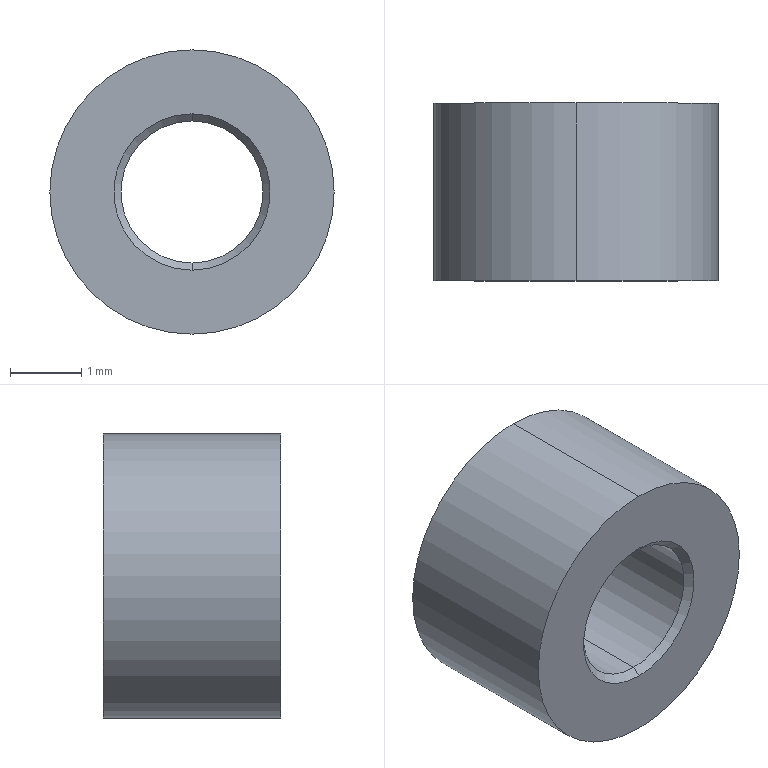Part | SolidWorks | features Chamfer 1, Extrusion 1 | 1 solid | 10 faces | box 4 x 2.5 x 4 mm | volume 23.497 mm3 | cone 4 | cylinder 4 | plane 2 | commonest cylinder face diameters 2 x2 4 x2
STEP:
#1=CARTESIAN_POINT('',(0.,2.4,-1.));
#2=VERTEX_POINT('',#1);
#3=CARTESIAN_POINT('',(0.,2.4,1.));
#4=VERTEX_POINT('',#3);
#5=CARTESIAN_POINT('',(0.,2.4,0.));
#6=DIRECTION('',(0.,1.,0.));
#7=DIRECTION('',(0.,0.,1.));
#8=AXIS2_PLACEMENT_3D('',#5,#6,#7);
#9=CIRCLE('',#8,1.);
#10=EDGE_CURVE('',#2,#4,#9,.T.);
#11=ORIENTED_EDGE('',*,*,#10,.F.);
#12=CARTESIAN_POINT('',(0.,2.5,-1.1));
#13=VERTEX_POINT('',#12);
#14=CARTESIAN_POINT('',(0.,2.4,-1.));
#15=DIRECTION('',(0.,0.7071,-0.7071));
#16=VECTOR('',#15,1000.);
#17=LINE('',#14,#16);
#18=EDGE_CURVE('',#2,#13,#17,.T.);
#19=ORIENTED_EDGE('',*,*,#18,.T.);
#20=CARTESIAN_POINT('',(0.,2.5,1.1));
#21=VERTEX_POINT('',#20);
#22=CARTESIAN_POINT('',(0.,2.5,0.));
#23=DIRECTION('',(0.,-1.,0.));
#24=DIRECTION('',(0.,0.,1.));
#25=AXIS2_PLACEMENT_3D('',#22,#23,#24);
#26=CIRCLE('',#25,1.1);
#27=EDGE_CURVE('',#21,#13,#26,.T.);
#28=ORIENTED_EDGE('',*,*,#27,.F.);
#29=CARTESIAN_POINT('',(0.,2.4,1.));
#30=DIRECTION('',(0.,0.7071,0.7071));
#31=VECTOR('',#30,1000.);
#32=LINE('',#29,#31);
#33=EDGE_CURVE('',#4,#21,#32,.T.);
#34=ORIENTED_EDGE('',*,*,#33,.F.);
#35=EDGE_LOOP('',(#11,#19,#28,#34));
#36=FACE_OUTER_BOUND('',#35,.T.);
#37=CARTESIAN_POINT('',(0.,2.4,0.));
#38=DIRECTION('',(0.,1.,0.));
#39=DIRECTION('',(0.,0.,1.));
#40=AXIS2_PLACEMENT_3D('',#37,#38,#39);
#41=CONICAL_SURFACE('',#40,1.,0.7854);
#42=ADVANCED_FACE('',(#36),#41,.F.);
#43=CARTESIAN_POINT('',(0.,0.1,1.));
#44=VERTEX_POINT('',#43);
#45=CARTESIAN_POINT('',(0.,0.1,-1.));
#46=VERTEX_POINT('',#45);
#47=CARTESIAN_POINT('',(0.,0.1,0.));
#48=DIRECTION('',(0.,-1.,0.));
#49=DIRECTION('',(0.,0.,1.));
#50=AXIS2_PLACEMENT_3D('',#47,#48,#49);
#51=CIRCLE('',#50,1.);
#52=EDGE_CURVE('',#44,#46,#51,.T.);
#53=ORIENTED_EDGE('',*,*,#52,.F.);
#54=CARTESIAN_POINT('',(0.,0.,1.1));
#55=VERTEX_POINT('',#54);
#56=CARTESIAN_POINT('',(0.,0.,1.1));
#57=DIRECTION('',(0.,-0.7071,0.7071));
#58=VECTOR('',#57,1000.);
#59=LINE('',#56,#58);
#60=EDGE_CURVE('',#44,#55,#59,.T.);
#61=ORIENTED_EDGE('',*,*,#60,.T.);
#62=CARTESIAN_POINT('',(0.,0.,-1.1));
#63=VERTEX_POINT('',#62);
#64=CARTESIAN_POINT('',(0.,0.,0.));
#65=DIRECTION('',(0.,1.,0.));
#66=DIRECTION('',(0.,0.,1.));
#67=AXIS2_PLACEMENT_3D('',#64,#65,#66);
#68=CIRCLE('',#67,1.1);
#69=EDGE_CURVE('',#63,#55,#68,.T.);
#70=ORIENTED_EDGE('',*,*,#69,.F.);
#71=CARTESIAN_POINT('',(0.,0.,-1.1));
#72=DIRECTION('',(0.,-0.7071,-0.7071));
#73=VECTOR('',#72,1000.);
#74=LINE('',#71,#73);
#75=EDGE_CURVE('',#46,#63,#74,.T.);
#76=ORIENTED_EDGE('',*,*,#75,.F.);
#77=EDGE_LOOP('',(#53,#61,#70,#76));
#78=FACE_OUTER_BOUND('',#77,.T.);
#79=CARTESIAN_POINT('',(0.,0.,0.));
#80=DIRECTION('',(0.,-1.,0.));
#81=DIRECTION('',(0.,0.,-1.));
#82=AXIS2_PLACEMENT_3D('',#79,#80,#81);
#83=CONICAL_SURFACE('',#82,1.1,0.7854);
#84=ADVANCED_FACE('',(#78),#83,.F.);
#85=ORIENTED_EDGE('',*,*,#10,.T.);
#86=CARTESIAN_POINT('',(0.,2.5,1.));
#87=DIRECTION('',(0.,-1.,0.));
#88=VECTOR('',#87,1000.);
#89=LINE('',#86,#88);
#90=EDGE_CURVE('',#4,#44,#89,.T.);
#91=ORIENTED_EDGE('',*,*,#90,.T.);
#92=ORIENTED_EDGE('',*,*,#52,.T.);
#93=CARTESIAN_POINT('',(0.,2.5,-1.));
#94=DIRECTION('',(0.,-1.,0.));
#95=VECTOR('',#94,1000.);
#96=LINE('',#93,#95);
#97=EDGE_CURVE('',#2,#46,#96,.T.);
#98=ORIENTED_EDGE('',*,*,#97,.F.);
#99=EDGE_LOOP('',(#85,#91,#92,#98));
#100=FACE_OUTER_BOUND('',#99,.T.);
#101=CARTESIAN_POINT('',(0.,2.5,0.));
#102=DIRECTION('',(0.,-1.,0.));
#103=DIRECTION('',(0.,0.,-1.));
#104=AXIS2_PLACEMENT_3D('',#101,#102,#103);
#105=CYLINDRICAL_SURFACE('',#104,1.);
#106=ADVANCED_FACE('',(#100),#105,.F.);
#107=CARTESIAN_POINT('',(0.,2.5,2.));
#108=VERTEX_POINT('',#107);
#109=CARTESIAN_POINT('',(0.,2.5,-2.));
#110=VERTEX_POINT('',#109);
#111=CARTESIAN_POINT('',(0.,2.5,0.));
#112=DIRECTION('',(0.,1.,0.));
#113=DIRECTION('',(0.,0.,1.));
#114=AXIS2_PLACEMENT_3D('',#111,#112,#113);
#115=CIRCLE('',#114,2.);
#116=EDGE_CURVE('',#108,#110,#115,.T.);
#117=ORIENTED_EDGE('',*,*,#116,.F.);
#118=CARTESIAN_POINT('',(0.,0.,2.));
#119=VERTEX_POINT('',#118);
#120=CARTESIAN_POINT('',(0.,2.5,2.));
#121=DIRECTION('',(0.,-1.,0.));
#122=VECTOR('',#121,1000.);
#123=LINE('',#120,#122);
#124=EDGE_CURVE('',#108,#119,#123,.T.);
#125=ORIENTED_EDGE('',*,*,#124,.T.);
#126=CARTESIAN_POINT('',(0.,0.,-2.));
#127=VERTEX_POINT('',#126);
#128=CARTESIAN_POINT('',(0.,0.,0.));
#129=DIRECTION('',(0.,1.,0.));
#130=DIRECTION('',(0.,0.,1.));
#131=AXIS2_PLACEMENT_3D('',#128,#129,#130);
#132=CIRCLE('',#131,2.);
#133=EDGE_CURVE('',#119,#127,#132,.T.);
#134=ORIENTED_EDGE('',*,*,#133,.T.);
#135=CARTESIAN_POINT('',(0.,2.5,-2.));
#136=DIRECTION('',(0.,-1.,0.));
#137=VECTOR('',#136,1000.);
#138=LINE('',#135,#137);
#139=EDGE_CURVE('',#110,#127,#138,.T.);
#140=ORIENTED_EDGE('',*,*,#139,.F.);
#141=EDGE_LOOP('',(#117,#125,#134,#140));
#142=FACE_OUTER_BOUND('',#141,.T.);
#143=CARTESIAN_POINT('',(0.,2.5,0.));
#144=DIRECTION('',(0.,-1.,0.));
#145=DIRECTION('',(0.,0.,-1.));
#146=AXIS2_PLACEMENT_3D('',#143,#144,#145);
#147=CYLINDRICAL_SURFACE('',#146,2.);
#148=ADVANCED_FACE('',(#142),#147,.T.);
#149=ORIENTED_EDGE('',*,*,#27,.T.);
#150=CARTESIAN_POINT('',(0.,2.5,0.));
#151=DIRECTION('',(0.,-1.,0.));
#152=DIRECTION('',(0.,0.,1.));
#153=AXIS2_PLACEMENT_3D('',#150,#151,#152);
#154=CIRCLE('',#153,1.1);
#155=EDGE_CURVE('',#13,#21,#154,.T.);
#156=ORIENTED_EDGE('',*,*,#155,.T.);
#157=EDGE_LOOP('',(#149,#156));
#158=FACE_BOUND('',#157,.T.);
#159=CARTESIAN_POINT('',(0.,2.5,0.));
#160=DIRECTION('',(0.,1.,0.));
#161=DIRECTION('',(0.,0.,1.));
#162=AXIS2_PLACEMENT_3D('',#159,#160,#161);
#163=CIRCLE('',#162,2.);
#164=EDGE_CURVE('',#110,#108,#163,.T.);
#165=ORIENTED_EDGE('',*,*,#164,.T.);
#166=ORIENTED_EDGE('',*,*,#116,.T.);
#167=EDGE_LOOP('',(#165,#166));
#168=FACE_OUTER_BOUND('',#167,.T.);
#169=CARTESIAN_POINT('',(0.,2.5,0.));
#170=DIRECTION('',(0.,1.,0.));
#171=DIRECTION('',(0.,0.,1.));
#172=AXIS2_PLACEMENT_3D('',#169,#170,#171);
#173=PLANE('',#172);
#174=ADVANCED_FACE('',(#158,#168),#173,.T.);
#175=ORIENTED_EDGE('',*,*,#69,.T.);
#176=CARTESIAN_POINT('',(0.,0.,0.));
#177=DIRECTION('',(0.,1.,0.));
#178=DIRECTION('',(0.,0.,1.));
#179=AXIS2_PLACEMENT_3D('',#176,#177,#178);
#180=CIRCLE('',#179,1.1);
#181=EDGE_CURVE('',#55,#63,#180,.T.);
#182=ORIENTED_EDGE('',*,*,#181,.T.);
#183=EDGE_LOOP('',(#175,#182));
#184=FACE_BOUND('',#183,.T.);
#185=CARTESIAN_POINT('',(0.,0.,0.));
#186=DIRECTION('',(0.,1.,0.));
#187=DIRECTION('',(0.,0.,1.));
#188=AXIS2_PLACEMENT_3D('',#185,#186,#187);
#189=CIRCLE('',#188,2.);
#190=EDGE_CURVE('',#127,#119,#189,.T.);
#191=ORIENTED_EDGE('',*,*,#190,.F.);
#192=ORIENTED_EDGE('',*,*,#133,.F.);
#193=EDGE_LOOP('',(#191,#192));
#194=FACE_OUTER_BOUND('',#193,.T.);
#195=CARTESIAN_POINT('',(0.,0.,0.));
#196=DIRECTION('',(0.,1.,0.));
#197=DIRECTION('',(0.,0.,1.));
#198=AXIS2_PLACEMENT_3D('',#195,#196,#197);
#199=PLANE('',#198);
#200=ADVANCED_FACE('',(#184,#194),#199,.F.);
#201=ORIENTED_EDGE('',*,*,#124,.F.);
#202=ORIENTED_EDGE('',*,*,#164,.F.);
#203=ORIENTED_EDGE('',*,*,#139,.T.);
#204=ORIENTED_EDGE('',*,*,#190,.T.);
#205=EDGE_LOOP('',(#201,#202,#203,#204));
#206=FACE_OUTER_BOUND('',#205,.T.);
#207=CARTESIAN_POINT('',(0.,2.5,0.));
#208=DIRECTION('',(0.,-1.,0.));
#209=DIRECTION('',(0.,0.,-1.));
#210=AXIS2_PLACEMENT_3D('',#207,#208,#209);
#211=CYLINDRICAL_SURFACE('',#210,2.);
#212=ADVANCED_FACE('',(#206),#211,.T.);
#213=ORIENTED_EDGE('',*,*,#90,.F.);
#214=CARTESIAN_POINT('',(0.,2.4,0.));
#215=DIRECTION('',(0.,1.,0.));
#216=DIRECTION('',(0.,0.,1.));
#217=AXIS2_PLACEMENT_3D('',#214,#215,#216);
#218=CIRCLE('',#217,1.);
#219=EDGE_CURVE('',#4,#2,#218,.T.);
#220=ORIENTED_EDGE('',*,*,#219,.T.);
#221=ORIENTED_EDGE('',*,*,#97,.T.);
#222=CARTESIAN_POINT('',(0.,0.1,0.));
#223=DIRECTION('',(0.,-1.,0.));
#224=DIRECTION('',(0.,0.,1.));
#225=AXIS2_PLACEMENT_3D('',#222,#223,#224);
#226=CIRCLE('',#225,1.);
#227=EDGE_CURVE('',#46,#44,#226,.T.);
#228=ORIENTED_EDGE('',*,*,#227,.T.);
#229=EDGE_LOOP('',(#213,#220,#221,#228));
#230=FACE_OUTER_BOUND('',#229,.T.);
#231=CARTESIAN_POINT('',(0.,2.5,0.));
#232=DIRECTION('',(0.,-1.,0.));
#233=DIRECTION('',(0.,0.,-1.));
#234=AXIS2_PLACEMENT_3D('',#231,#232,#233);
#235=CYLINDRICAL_SURFACE('',#234,1.);
#236=ADVANCED_FACE('',(#230),#235,.F.);
#237=ORIENTED_EDGE('',*,*,#60,.F.);
#238=ORIENTED_EDGE('',*,*,#227,.F.);
#239=ORIENTED_EDGE('',*,*,#75,.T.);
#240=ORIENTED_EDGE('',*,*,#181,.F.);
#241=EDGE_LOOP('',(#237,#238,#239,#240));
#242=FACE_OUTER_BOUND('',#241,.T.);
#243=CARTESIAN_POINT('',(0.,0.,0.));
#244=DIRECTION('',(0.,-1.,0.));
#245=DIRECTION('',(0.,0.,-1.));
#246=AXIS2_PLACEMENT_3D('',#243,#244,#245);
#247=CONICAL_SURFACE('',#246,1.1,0.7854);
#248=ADVANCED_FACE('',(#242),#247,.F.);
#249=ORIENTED_EDGE('',*,*,#18,.F.);
#250=ORIENTED_EDGE('',*,*,#219,.F.);
#251=ORIENTED_EDGE('',*,*,#33,.T.);
#252=ORIENTED_EDGE('',*,*,#155,.F.);
#253=EDGE_LOOP('',(#249,#250,#251,#252));
#254=FACE_OUTER_BOUND('',#253,.T.);
#255=CARTESIAN_POINT('',(0.,2.4,0.));
#256=DIRECTION('',(0.,1.,0.));
#257=DIRECTION('',(0.,0.,1.));
#258=AXIS2_PLACEMENT_3D('',#255,#256,#257);
#259=CONICAL_SURFACE('',#258,1.,0.7854);
#260=ADVANCED_FACE('',(#254),#259,.F.);
#261=CLOSED_SHELL('',(#42,#84,#106,#148,#174,#200,#212,#236,#248,#260));
#262=MANIFOLD_SOLID_BREP('',#261);
#263=CARTESIAN_POINT('',(0.,0.,0.));
#264=DIRECTION('',(0.,0.,1.));
#265=DIRECTION('',(1.,0.,0.));
#266=AXIS2_PLACEMENT_3D('',#263,#264,#265);
#267=(LENGTH_UNIT()NAMED_UNIT(*)SI_UNIT(.MILLI.,.METRE.));
#268=UNCERTAINTY_MEASURE_WITH_UNIT(LENGTH_MEASURE(0.00001),#267,'','');
#269=(NAMED_UNIT(*)PLANE_ANGLE_UNIT()SI_UNIT($,.RADIAN.));
#270=(NAMED_UNIT(*)SI_UNIT($,.STERADIAN.)SOLID_ANGLE_UNIT());
#271=(GEOMETRIC_REPRESENTATION_CONTEXT(3)GLOBAL_UNCERTAINTY_ASSIGNED_CONTEXT((#268))GLOBAL_UNIT_ASSIGNED_CONTEXT((#267,#269,#270))REPRESENTATION_CONTEXT('',''));
#272=ADVANCED_BREP_SHAPE_REPRESENTATION('',(#262,#266),#271);